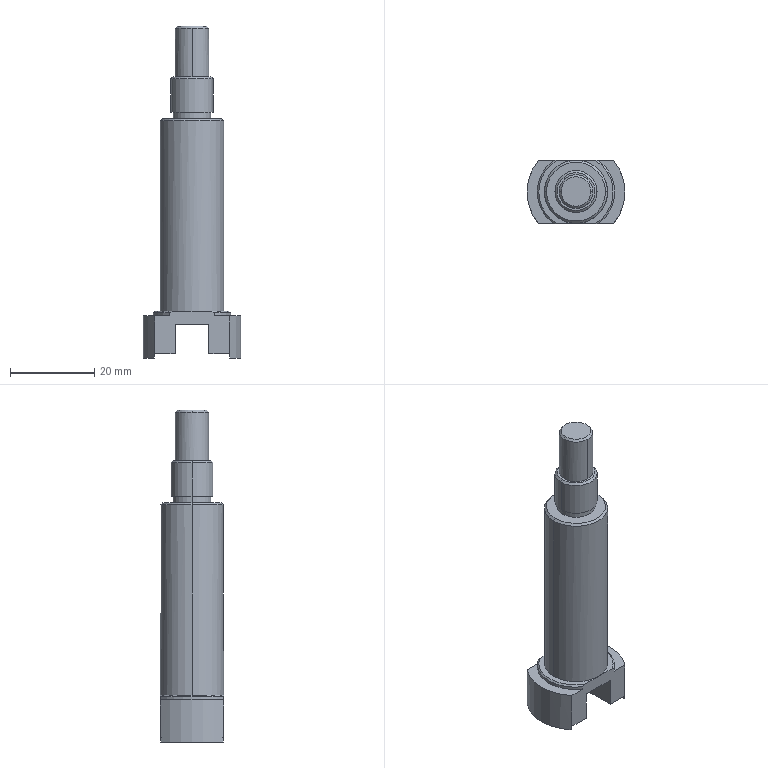Part | NX | 1 solid | 52 faces | box 23.26 x 15 x 78.8 mm | volume 11720 mm3 | plane 19 | cone 17 | cylinder 16 | commonest cylinder face diameters 2.5 x4 8 x2 9 x2 10 x2 15 x2 18.4 x2
STEP:
#1=CARTESIAN_POINT('',(4.5,0.,10.));
#2=VERTEX_POINT('',#1);
#3=CARTESIAN_POINT('',(-4.5,0.,10.));
#4=VERTEX_POINT('',#3);
#5=CARTESIAN_POINT('',(0.,0.,10.));
#6=DIRECTION('',(0.,0.,-1.));
#7=DIRECTION('',(1.,0.,0.));
#8=AXIS2_PLACEMENT_3D('',#5,#6,#7);
#9=CIRCLE('',#8,4.5);
#10=EDGE_CURVE('',#2,#4,#9,.T.);
#11=ORIENTED_EDGE('',*,*,#10,.F.);
#12=CARTESIAN_POINT('',(0.,0.,10.));
#13=DIRECTION('',(0.,0.,-1.));
#14=DIRECTION('',(1.,0.,0.));
#15=AXIS2_PLACEMENT_3D('',#12,#13,#14);
#16=CIRCLE('',#15,4.5);
#17=EDGE_CURVE('',#4,#2,#16,.T.);
#18=ORIENTED_EDGE('',*,*,#17,.F.);
#19=EDGE_LOOP('',(#11,#18));
#20=FACE_BOUND('',#19,.T.);
#21=CARTESIAN_POINT('',(0.,-4.,10.));
#22=VERTEX_POINT('',#21);
#23=CARTESIAN_POINT('',(0.,4.,10.));
#24=VERTEX_POINT('',#23);
#25=CARTESIAN_POINT('',(0.,0.,10.));
#26=DIRECTION('',(0.,0.,1.));
#27=DIRECTION('',(0.,-1.,0.));
#28=AXIS2_PLACEMENT_3D('',#25,#26,#27);
#29=CIRCLE('',#28,4.);
#30=EDGE_CURVE('',#22,#24,#29,.T.);
#31=ORIENTED_EDGE('',*,*,#30,.F.);
#32=CARTESIAN_POINT('',(0.,0.,10.));
#33=DIRECTION('',(0.,0.,1.));
#34=DIRECTION('',(0.,-1.,0.));
#35=AXIS2_PLACEMENT_3D('',#32,#33,#34);
#36=CIRCLE('',#35,4.);
#37=EDGE_CURVE('',#24,#22,#36,.T.);
#38=ORIENTED_EDGE('',*,*,#37,.F.);
#39=EDGE_LOOP('',(#31,#38));
#40=FACE_BOUND('',#39,.T.);
#41=CARTESIAN_POINT('',(0.,0.,10.));
#42=DIRECTION('',(0.,0.,1.));
#43=DIRECTION('',(1.,0.,0.));
#44=AXIS2_PLACEMENT_3D('',#41,#42,#43);
#45=PLANE('',#44);
#46=ADVANCED_FACE('',(#20,#40),#45,.T.);
#47=ORIENTED_EDGE('',*,*,#10,.T.);
#48=CARTESIAN_POINT('',(-5.,0.,9.5));
#49=VERTEX_POINT('',#48);
#50=CARTESIAN_POINT('',(-4.75,0.,9.75));
#51=DIRECTION('',(-0.7071,0.,-0.7071));
#52=VECTOR('',#51,1000.);
#53=LINE('',#50,#52);
#54=EDGE_CURVE('',#49,#4,#53,.F.);
#55=ORIENTED_EDGE('',*,*,#54,.F.);
#56=CARTESIAN_POINT('',(5.,0.,9.5));
#57=VERTEX_POINT('',#56);
#58=CARTESIAN_POINT('',(0.,0.,9.5));
#59=DIRECTION('',(0.,0.,-1.));
#60=DIRECTION('',(1.,0.,0.));
#61=AXIS2_PLACEMENT_3D('',#58,#59,#60);
#62=CIRCLE('',#61,5.);
#63=EDGE_CURVE('',#57,#49,#62,.T.);
#64=ORIENTED_EDGE('',*,*,#63,.F.);
#65=CARTESIAN_POINT('',(4.75,0.,9.75));
#66=DIRECTION('',(0.7071,0.,-0.7071));
#67=VECTOR('',#66,1000.);
#68=LINE('',#65,#67);
#69=EDGE_CURVE('',#57,#2,#68,.F.);
#70=ORIENTED_EDGE('',*,*,#69,.T.);
#71=EDGE_LOOP('',(#47,#55,#64,#70));
#72=FACE_BOUND('',#71,.T.);
#73=CARTESIAN_POINT('',(0.,0.,9.75));
#74=DIRECTION('',(0.,0.,-1.));
#75=DIRECTION('',(-1.,0.,0.));
#76=AXIS2_PLACEMENT_3D('',#73,#74,#75);
#77=CONICAL_SURFACE('',#76,4.75,0.7854);
#78=ADVANCED_FACE('',(#72),#77,.T.);
#79=ORIENTED_EDGE('',*,*,#30,.T.);
#80=CARTESIAN_POINT('',(0.,4.,21.5));
#81=VERTEX_POINT('',#80);
#82=CARTESIAN_POINT('',(0.,4.,10.));
#83=DIRECTION('',(0.,0.,1.));
#84=VECTOR('',#83,1000.);
#85=LINE('',#82,#84);
#86=EDGE_CURVE('',#24,#81,#85,.T.);
#87=ORIENTED_EDGE('',*,*,#86,.T.);
#88=CARTESIAN_POINT('',(4.,0.,21.5));
#89=VERTEX_POINT('',#88);
#90=CARTESIAN_POINT('',(0.,0.,21.5));
#91=DIRECTION('',(0.,0.,-1.));
#92=DIRECTION('',(0.,1.,0.));
#93=AXIS2_PLACEMENT_3D('',#90,#91,#92);
#94=CIRCLE('',#93,4.);
#95=EDGE_CURVE('',#81,#89,#94,.T.);
#96=ORIENTED_EDGE('',*,*,#95,.T.);
#97=CARTESIAN_POINT('',(0.,-4.,21.5));
#98=VERTEX_POINT('',#97);
#99=CARTESIAN_POINT('',(0.,0.,21.5));
#100=DIRECTION('',(0.,0.,-1.));
#101=DIRECTION('',(0.,1.,0.));
#102=AXIS2_PLACEMENT_3D('',#99,#100,#101);
#103=CIRCLE('',#102,4.);
#104=EDGE_CURVE('',#89,#98,#103,.T.);
#105=ORIENTED_EDGE('',*,*,#104,.T.);
#106=CARTESIAN_POINT('',(0.,-4.,10.));
#107=DIRECTION('',(0.,0.,1.));
#108=VECTOR('',#107,1000.);
#109=LINE('',#106,#108);
#110=EDGE_CURVE('',#22,#98,#109,.T.);
#111=ORIENTED_EDGE('',*,*,#110,.F.);
#112=EDGE_LOOP('',(#79,#87,#96,#105,#111));
#113=FACE_BOUND('',#112,.T.);
#114=CARTESIAN_POINT('',(0.,0.,10.));
#115=DIRECTION('',(0.,0.,1.));
#116=DIRECTION('',(0.,1.,0.));
#117=AXIS2_PLACEMENT_3D('',#114,#115,#116);
#118=CYLINDRICAL_SURFACE('',#117,4.);
#119=ADVANCED_FACE('',(#113),#118,.T.);
#120=CARTESIAN_POINT('',(4.8,7.5,-50.8));
#121=VERTEX_POINT('',#120);
#122=CARTESIAN_POINT('',(8.2,7.5,-50.8));
#123=VERTEX_POINT('',#122);
#124=CARTESIAN_POINT('',(6.5,7.5,-50.8));
#125=DIRECTION('',(0.,1.,0.));
#126=DIRECTION('',(1.,0.,0.));
#127=AXIS2_PLACEMENT_3D('',#124,#125,#126);
#128=CIRCLE('',#127,1.7);
#129=EDGE_CURVE('',#121,#123,#128,.T.);
#130=ORIENTED_EDGE('',*,*,#129,.T.);
#131=CARTESIAN_POINT('',(7.75,7.24,-50.8));
#132=VERTEX_POINT('',#131);
#133=CARTESIAN_POINT('',(7.75,7.24,-50.8));
#134=DIRECTION('',(0.866,0.5,0.));
#135=VECTOR('',#134,1000.);
#136=LINE('',#133,#135);
#137=EDGE_CURVE('',#132,#123,#136,.T.);
#138=ORIENTED_EDGE('',*,*,#137,.F.);
#139=CARTESIAN_POINT('',(5.25,7.24,-50.8));
#140=VERTEX_POINT('',#139);
#141=CARTESIAN_POINT('',(6.5,7.24,-50.8));
#142=DIRECTION('',(0.,1.,0.));
#143=DIRECTION('',(1.,0.,0.));
#144=AXIS2_PLACEMENT_3D('',#141,#142,#143);
#145=CIRCLE('',#144,1.25);
#146=EDGE_CURVE('',#140,#132,#145,.T.);
#147=ORIENTED_EDGE('',*,*,#146,.F.);
#148=CARTESIAN_POINT('',(5.25,7.24,-50.8));
#149=DIRECTION('',(-0.866,0.5,0.));
#150=VECTOR('',#149,1000.);
#151=LINE('',#148,#150);
#152=EDGE_CURVE('',#140,#121,#151,.T.);
#153=ORIENTED_EDGE('',*,*,#152,.T.);
#154=EDGE_LOOP('',(#130,#138,#147,#153));
#155=FACE_BOUND('',#154,.T.);
#156=CARTESIAN_POINT('',(6.5,7.24,-50.8));
#157=DIRECTION('',(0.,1.,0.));
#158=DIRECTION('',(1.,0.,0.));
#159=AXIS2_PLACEMENT_3D('',#156,#157,#158);
#160=CONICAL_SURFACE('',#159,1.25,1.047);
#161=ADVANCED_FACE('',(#155),#160,.F.);
#162=ORIENTED_EDGE('',*,*,#63,.T.);
#163=CARTESIAN_POINT('',(-5.,0.,1.5));
#164=VERTEX_POINT('',#163);
#165=CARTESIAN_POINT('',(-5.,0.,0.));
#166=DIRECTION('',(0.,0.,1.));
#167=VECTOR('',#166,1000.);
#168=LINE('',#165,#167);
#169=EDGE_CURVE('',#164,#49,#168,.T.);
#170=ORIENTED_EDGE('',*,*,#169,.F.);
#171=CARTESIAN_POINT('',(5.,0.,1.5));
#172=VERTEX_POINT('',#171);
#173=CARTESIAN_POINT('',(0.,0.,1.5));
#174=DIRECTION('',(0.,0.,1.));
#175=DIRECTION('',(1.,0.,0.));
#176=AXIS2_PLACEMENT_3D('',#173,#174,#175);
#177=CIRCLE('',#176,5.);
#178=EDGE_CURVE('',#164,#172,#177,.T.);
#179=ORIENTED_EDGE('',*,*,#178,.T.);
#180=CARTESIAN_POINT('',(5.,0.,0.));
#181=DIRECTION('',(0.,0.,1.));
#182=VECTOR('',#181,1000.);
#183=LINE('',#180,#182);
#184=EDGE_CURVE('',#172,#57,#183,.T.);
#185=ORIENTED_EDGE('',*,*,#184,.T.);
#186=EDGE_LOOP('',(#162,#170,#179,#185));
#187=FACE_BOUND('',#186,.T.);
#188=CARTESIAN_POINT('',(0.,0.,0.));
#189=DIRECTION('',(0.,0.,1.));
#190=DIRECTION('',(1.,0.,0.));
#191=AXIS2_PLACEMENT_3D('',#188,#189,#190);
#192=CYLINDRICAL_SURFACE('',#191,5.);
#193=ADVANCED_FACE('',(#187),#192,.T.);
#194=CARTESIAN_POINT('',(7.5,0.,-0.5));
#195=VERTEX_POINT('',#194);
#196=CARTESIAN_POINT('',(-7.5,0.,-0.5));
#197=VERTEX_POINT('',#196);
#198=CARTESIAN_POINT('',(0.,0.,-0.5));
#199=DIRECTION('',(0.,0.,-1.));
#200=DIRECTION('',(-1.,0.,0.));
#201=AXIS2_PLACEMENT_3D('',#198,#199,#200);
#202=CIRCLE('',#201,7.5);
#203=EDGE_CURVE('',#195,#197,#202,.T.);
#204=ORIENTED_EDGE('',*,*,#203,.F.);
#205=CARTESIAN_POINT('',(7.,0.,0.));
#206=VERTEX_POINT('',#205);
#207=CARTESIAN_POINT('',(7.25,0.,-0.25));
#208=DIRECTION('',(0.7071,0.,-0.7071));
#209=VECTOR('',#208,1000.);
#210=LINE('',#207,#209);
#211=EDGE_CURVE('',#206,#195,#210,.T.);
#212=ORIENTED_EDGE('',*,*,#211,.F.);
#213=CARTESIAN_POINT('',(-7.,0.,0.));
#214=VERTEX_POINT('',#213);
#215=CARTESIAN_POINT('',(0.,0.,0.));
#216=DIRECTION('',(0.,0.,-1.));
#217=DIRECTION('',(-1.,0.,0.));
#218=AXIS2_PLACEMENT_3D('',#215,#216,#217);
#219=CIRCLE('',#218,7.);
#220=EDGE_CURVE('',#206,#214,#219,.T.);
#221=ORIENTED_EDGE('',*,*,#220,.T.);
#222=CARTESIAN_POINT('',(-7.25,0.,-0.25));
#223=DIRECTION('',(-0.7071,0.,-0.7071));
#224=VECTOR('',#223,1000.);
#225=LINE('',#222,#224);
#226=EDGE_CURVE('',#214,#197,#225,.T.);
#227=ORIENTED_EDGE('',*,*,#226,.T.);
#228=EDGE_LOOP('',(#204,#212,#221,#227));
#229=FACE_BOUND('',#228,.T.);
#230=CARTESIAN_POINT('',(0.,0.,-0.25));
#231=DIRECTION('',(0.,0.,-1.));
#232=DIRECTION('',(-1.,0.,0.));
#233=AXIS2_PLACEMENT_3D('',#230,#231,#232);
#234=CONICAL_SURFACE('',#233,7.25,0.7854);
#235=ADVANCED_FACE('',(#229),#234,.T.);
#236=CARTESIAN_POINT('',(-4.,0.,21.5));
#237=VERTEX_POINT('',#236);
#238=CARTESIAN_POINT('',(0.,0.,21.5));
#239=DIRECTION('',(0.,0.,-1.));
#240=DIRECTION('',(0.,1.,0.));
#241=AXIS2_PLACEMENT_3D('',#238,#239,#240);
#242=CIRCLE('',#241,4.);
#243=EDGE_CURVE('',#237,#81,#242,.T.);
#244=ORIENTED_EDGE('',*,*,#243,.F.);
#245=CARTESIAN_POINT('',(-3.5,0.,22.));
#246=VERTEX_POINT('',#245);
#247=CARTESIAN_POINT('',(-3.75,0.,21.75));
#248=DIRECTION('',(-0.7071,0.,-0.7071));
#249=VECTOR('',#248,1000.);
#250=LINE('',#247,#249);
#251=EDGE_CURVE('',#237,#246,#250,.F.);
#252=ORIENTED_EDGE('',*,*,#251,.T.);
#253=CARTESIAN_POINT('',(3.5,0.,22.));
#254=VERTEX_POINT('',#253);
#255=CARTESIAN_POINT('',(0.,0.,22.));
#256=DIRECTION('',(0.,0.,-1.));
#257=DIRECTION('',(0.,-1.,0.));
#258=AXIS2_PLACEMENT_3D('',#255,#256,#257);
#259=CIRCLE('',#258,3.5);
#260=EDGE_CURVE('',#246,#254,#259,.T.);
#261=ORIENTED_EDGE('',*,*,#260,.T.);
#262=CARTESIAN_POINT('',(3.75,0.,21.75));
#263=DIRECTION('',(0.7071,0.,-0.7071));
#264=VECTOR('',#263,1000.);
#265=LINE('',#262,#264);
#266=EDGE_CURVE('',#89,#254,#265,.F.);
#267=ORIENTED_EDGE('',*,*,#266,.F.);
#268=ORIENTED_EDGE('',*,*,#95,.F.);
#269=EDGE_LOOP('',(#244,#252,#261,#267,#268));
#270=FACE_BOUND('',#269,.T.);
#271=CARTESIAN_POINT('',(0.,0.,21.75));
#272=DIRECTION('',(0.,0.,-1.));
#273=DIRECTION('',(-1.,0.,0.));
#274=AXIS2_PLACEMENT_3D('',#271,#272,#273);
#275=CONICAL_SURFACE('',#274,3.75,0.7854);
#276=ADVANCED_FACE('',(#270),#275,.T.);
#277=ORIENTED_EDGE('',*,*,#203,.T.);
#278=CARTESIAN_POINT('',(-7.5,0.,-45.7));
#279=VERTEX_POINT('',#278);
#280=CARTESIAN_POINT('',(-7.5,0.,2.34));
#281=DIRECTION('',(0.,0.,-1.));
#282=VECTOR('',#281,1000.);
#283=LINE('',#280,#282);
#284=EDGE_CURVE('',#279,#197,#283,.F.);
#285=ORIENTED_EDGE('',*,*,#284,.F.);
#286=CARTESIAN_POINT('',(0.,-7.5,-45.7));
#287=VERTEX_POINT('',#286);
#288=CARTESIAN_POINT('',(0.,0.,-45.7));
#289=DIRECTION('',(0.,0.,1.));
#290=DIRECTION('',(-1.,0.,0.));
#291=AXIS2_PLACEMENT_3D('',#288,#289,#290);
#292=CIRCLE('',#291,7.5);
#293=EDGE_CURVE('',#279,#287,#292,.T.);
#294=ORIENTED_EDGE('',*,*,#293,.T.);
#295=CARTESIAN_POINT('',(7.5,0.,-45.7));
#296=VERTEX_POINT('',#295);
#297=CARTESIAN_POINT('',(0.,0.,-45.7));
#298=DIRECTION('',(0.,0.,1.));
#299=DIRECTION('',(0.,-1.,0.));
#300=AXIS2_PLACEMENT_3D('',#297,#298,#299);
#301=CIRCLE('',#300,7.5);
#302=EDGE_CURVE('',#287,#296,#301,.T.);
#303=ORIENTED_EDGE('',*,*,#302,.T.);
#304=CARTESIAN_POINT('',(7.5,0.,2.34));
#305=DIRECTION('',(0.,0.,-1.));
#306=VECTOR('',#305,1000.);
#307=LINE('',#304,#306);
#308=EDGE_CURVE('',#296,#195,#307,.F.);
#309=ORIENTED_EDGE('',*,*,#308,.T.);
#310=EDGE_LOOP('',(#277,#285,#294,#303,#309));
#311=FACE_BOUND('',#310,.T.);
#312=CARTESIAN_POINT('',(0.,0.,2.34));
#313=DIRECTION('',(0.,0.,-1.));
#314=DIRECTION('',(1.,0.,0.));
#315=AXIS2_PLACEMENT_3D('',#312,#313,#314);
#316=CYLINDRICAL_SURFACE('',#315,7.5);
#317=ADVANCED_FACE('',(#311),#316,.T.);
#318=CARTESIAN_POINT('',(-4.651,7.5,-45.7));
#319=VERTEX_POINT('',#318);
#320=CARTESIAN_POINT('',(0.,7.5,-45.7));
#321=VERTEX_POINT('',#320);
#322=CARTESIAN_POINT('',(0.,7.5,-45.7));
#323=DIRECTION('',(1.,0.,0.));
#324=VECTOR('',#323,1000.);
#325=LINE('',#322,#324);
#326=EDGE_CURVE('',#319,#321,#325,.T.);
#327=ORIENTED_EDGE('',*,*,#326,.F.);
#328=CARTESIAN_POINT('',(-8.825,0.,-45.7));
#329=VERTEX_POINT('',#328);
#330=CARTESIAN_POINT('',(0.,0.,-45.7));
#331=DIRECTION('',(0.,0.,-1.));
#332=DIRECTION('',(-1.,0.,0.));
#333=AXIS2_PLACEMENT_3D('',#330,#331,#332);
#334=CIRCLE('',#333,8.825);
#335=EDGE_CURVE('',#329,#319,#334,.T.);
#336=ORIENTED_EDGE('',*,*,#335,.F.);
#337=CARTESIAN_POINT('',(-4.651,-7.5,-45.7));
#338=VERTEX_POINT('',#337);
#339=CARTESIAN_POINT('',(0.,0.,-45.7));
#340=DIRECTION('',(0.,0.,-1.));
#341=DIRECTION('',(-1.,0.,0.));
#342=AXIS2_PLACEMENT_3D('',#339,#340,#341);
#343=CIRCLE('',#342,8.825);
#344=EDGE_CURVE('',#338,#329,#343,.T.);
#345=ORIENTED_EDGE('',*,*,#344,.F.);
#346=CARTESIAN_POINT('',(0.,-7.5,-45.7));
#347=DIRECTION('',(-1.,0.,0.));
#348=VECTOR('',#347,1000.);
#349=LINE('',#346,#348);
#350=EDGE_CURVE('',#287,#338,#349,.T.);
#351=ORIENTED_EDGE('',*,*,#350,.F.);
#352=ORIENTED_EDGE('',*,*,#293,.F.);
#353=CARTESIAN_POINT('',(0.,0.,-45.7));
#354=DIRECTION('',(0.,0.,1.));
#355=DIRECTION('',(-1.,0.,0.));
#356=AXIS2_PLACEMENT_3D('',#353,#354,#355);
#357=CIRCLE('',#356,7.5);
#358=EDGE_CURVE('',#321,#279,#357,.T.);
#359=ORIENTED_EDGE('',*,*,#358,.F.);
#360=EDGE_LOOP('',(#327,#336,#345,#351,#352,#359));
#361=FACE_BOUND('',#360,.T.);
#362=CARTESIAN_POINT('',(0.,0.,-45.7));
#363=DIRECTION('',(0.,0.,1.));
#364=DIRECTION('',(1.,0.,0.));
#365=AXIS2_PLACEMENT_3D('',#362,#363,#364);
#366=PLANE('',#365);
#367=ADVANCED_FACE('',(#361),#366,.T.);
#368=CARTESIAN_POINT('',(4.,7.5,-55.8));
#369=VERTEX_POINT('',#368);
#370=CARTESIAN_POINT('',(8.889,7.5,-55.8));
#371=VERTEX_POINT('',#370);
#372=CARTESIAN_POINT('',(0.,7.5,-55.8));
#373=DIRECTION('',(1.,0.,0.));
#374=VECTOR('',#373,1000.);
#375=LINE('',#372,#374);
#376=EDGE_CURVE('',#369,#371,#375,.T.);
#377=ORIENTED_EDGE('',*,*,#376,.F.);
#378=CARTESIAN_POINT('',(4.,7.5,-48.8));
#379=VERTEX_POINT('',#378);
#380=CARTESIAN_POINT('',(4.,7.5,0.));
#381=DIRECTION('',(0.,0.,-1.));
#382=VECTOR('',#381,1000.);
#383=LINE('',#380,#382);
#384=EDGE_CURVE('',#379,#369,#383,.T.);
#385=ORIENTED_EDGE('',*,*,#384,.F.);
#386=CARTESIAN_POINT('',(-4.,7.5,-48.8));
#387=VERTEX_POINT('',#386);
#388=CARTESIAN_POINT('',(0.,7.5,-48.8));
#389=DIRECTION('',(1.,0.,0.));
#390=VECTOR('',#389,1000.);
#391=LINE('',#388,#390);
#392=EDGE_CURVE('',#387,#379,#391,.T.);
#393=ORIENTED_EDGE('',*,*,#392,.F.);
#394=CARTESIAN_POINT('',(-4.,7.5,-55.8));
#395=VERTEX_POINT('',#394);
#396=CARTESIAN_POINT('',(-4.,7.5,0.));
#397=DIRECTION('',(0.,0.,1.));
#398=VECTOR('',#397,1000.);
#399=LINE('',#396,#398);
#400=EDGE_CURVE('',#395,#387,#399,.T.);
#401=ORIENTED_EDGE('',*,*,#400,.F.);
#402=CARTESIAN_POINT('',(-8.889,7.5,-55.8));
#403=VERTEX_POINT('',#402);
#404=CARTESIAN_POINT('',(0.,7.5,-55.8));
#405=DIRECTION('',(1.,0.,0.));
#406=VECTOR('',#405,1000.);
#407=LINE('',#404,#406);
#408=EDGE_CURVE('',#403,#395,#407,.T.);
#409=ORIENTED_EDGE('',*,*,#408,.F.);
#410=CARTESIAN_POINT('',(-8.889,7.5,-46.8));
#411=VERTEX_POINT('',#410);
#412=CARTESIAN_POINT('',(-8.889,7.5,0.));
#413=DIRECTION('',(0.,0.,-1.));
#414=VECTOR('',#413,1000.);
#415=LINE('',#412,#414);
#416=EDGE_CURVE('',#411,#403,#415,.T.);
#417=ORIENTED_EDGE('',*,*,#416,.F.);
#418=CARTESIAN_POINT('',(-5.328,7.5,-46.8));
#419=VERTEX_POINT('',#418);
#420=CARTESIAN_POINT('',(0.,7.5,-46.8));
#421=DIRECTION('',(-1.,0.,0.));
#422=VECTOR('',#421,1000.);
#423=LINE('',#420,#422);
#424=EDGE_CURVE('',#419,#411,#423,.T.);
#425=ORIENTED_EDGE('',*,*,#424,.F.);
#426=CARTESIAN_POINT('',(-5.328,7.5,-46.075));
#427=VERTEX_POINT('',#426);
#428=CARTESIAN_POINT('',(-5.328,7.5,-46.8));
#429=DIRECTION('',(0.,0.,1.));
#430=VECTOR('',#429,1000.);
#431=LINE('',#428,#430);
#432=EDGE_CURVE('',#419,#427,#431,.T.);
#433=ORIENTED_EDGE('',*,*,#432,.T.);
#434=CARTESIAN_POINT('',(-5.328,7.5,-46.075));
#435=CARTESIAN_POINT('',(-5.273,7.5,-46.043));
#436=CARTESIAN_POINT('',(-5.217,7.5,-46.011));
#437=CARTESIAN_POINT('',(-5.161,7.5,-45.979));
#438=CARTESIAN_POINT('',(-5.104,7.5,-45.947));
#439=CARTESIAN_POINT('',(-5.048,7.5,-45.916));
#440=CARTESIAN_POINT('',(-4.992,7.5,-45.884));
#441=CARTESIAN_POINT('',(-4.935,7.5,-45.853));
#442=CARTESIAN_POINT('',(-4.879,7.5,-45.822));
#443=CARTESIAN_POINT('',(-4.822,7.5,-45.791));
#444=CARTESIAN_POINT('',(-4.765,7.5,-45.761));
#445=CARTESIAN_POINT('',(-4.708,7.5,-45.73));
#446=CARTESIAN_POINT('',(-4.651,7.5,-45.7));
#447=B_SPLINE_CURVE_WITH_KNOTS('',3,(#434,#435,#436,#437,#438,#439,#440,#441,#442,#443,#444,#445,#446),.UNSPECIFIED.,.F.,.F.,(4,3,3,3,4),(0.,0.1932,0.3867,0.5804,0.7743),.UNSPECIFIED.);
#448=EDGE_CURVE('',#427,#319,#447,.T.);
#449=ORIENTED_EDGE('',*,*,#448,.T.);
#450=ORIENTED_EDGE('',*,*,#326,.T.);
#451=CARTESIAN_POINT('',(4.651,7.5,-45.7));
#452=VERTEX_POINT('',#451);
#453=CARTESIAN_POINT('',(0.,7.5,-45.7));
#454=DIRECTION('',(1.,0.,0.));
#455=VECTOR('',#454,1000.);
#456=LINE('',#453,#455);
#457=EDGE_CURVE('',#321,#452,#456,.T.);
#458=ORIENTED_EDGE('',*,*,#457,.T.);
#459=CARTESIAN_POINT('',(5.328,7.5,-46.075));
#460=VERTEX_POINT('',#459);
#461=CARTESIAN_POINT('',(4.651,7.5,-45.7));
#462=CARTESIAN_POINT('',(4.708,7.5,-45.73));
#463=CARTESIAN_POINT('',(4.765,7.5,-45.761));
#464=CARTESIAN_POINT('',(4.822,7.5,-45.791));
#465=CARTESIAN_POINT('',(4.879,7.5,-45.822));
#466=CARTESIAN_POINT('',(4.935,7.5,-45.853));
#467=CARTESIAN_POINT('',(4.992,7.5,-45.884));
#468=CARTESIAN_POINT('',(5.048,7.5,-45.916));
#469=CARTESIAN_POINT('',(5.104,7.5,-45.947));
#470=CARTESIAN_POINT('',(5.161,7.5,-45.979));
#471=CARTESIAN_POINT('',(5.217,7.5,-46.011));
#472=CARTESIAN_POINT('',(5.273,7.5,-46.043));
#473=CARTESIAN_POINT('',(5.328,7.5,-46.075));
#474=B_SPLINE_CURVE_WITH_KNOTS('',3,(#461,#462,#463,#464,#465,#466,#467,#468,#469,#470,#471,#472,#473),.UNSPECIFIED.,.F.,.F.,(4,3,3,3,4),(0.,0.1939,0.3875,0.581,0.7743),.UNSPECIFIED.);
#475=EDGE_CURVE('',#452,#460,#474,.T.);
#476=ORIENTED_EDGE('',*,*,#475,.T.);
#477=CARTESIAN_POINT('',(5.328,7.5,-46.8));
#478=VERTEX_POINT('',#477);
#479=CARTESIAN_POINT('',(5.328,7.5,-46.8));
#480=DIRECTION('',(0.,0.,1.));
#481=VECTOR('',#480,1000.);
#482=LINE('',#479,#481);
#483=EDGE_CURVE('',#478,#460,#482,.T.);
#484=ORIENTED_EDGE('',*,*,#483,.F.);
#485=CARTESIAN_POINT('',(8.889,7.5,-46.8));
#486=VERTEX_POINT('',#485);
#487=CARTESIAN_POINT('',(0.,7.5,-46.8));
#488=DIRECTION('',(1.,0.,0.));
#489=VECTOR('',#488,1000.);
#490=LINE('',#487,#489);
#491=EDGE_CURVE('',#478,#486,#490,.T.);
#492=ORIENTED_EDGE('',*,*,#491,.T.);
#493=CARTESIAN_POINT('',(8.889,7.5,0.));
#494=DIRECTION('',(0.,0.,-1.));
#495=VECTOR('',#494,1000.);
#496=LINE('',#493,#495);
#497=EDGE_CURVE('',#486,#371,#496,.T.);
#498=ORIENTED_EDGE('',*,*,#497,.T.);
#499=EDGE_LOOP('',(#377,#385,#393,#401,#409,#417,#425,#433,#449,#450,#458,#476,#484,#492,#498));
#500=FACE_BOUND('',#499,.T.);
#501=CARTESIAN_POINT('',(-8.2,7.5,-50.8));
#502=VERTEX_POINT('',#501);
#503=CARTESIAN_POINT('',(-4.8,7.5,-50.8));
#504=VERTEX_POINT('',#503);
#505=CARTESIAN_POINT('',(-6.5,7.5,-50.8));
#506=DIRECTION('',(0.,1.,0.));
#507=DIRECTION('',(1.,0.,0.));
#508=AXIS2_PLACEMENT_3D('',#505,#506,#507);
#509=CIRCLE('',#508,1.7);
#510=EDGE_CURVE('',#502,#504,#509,.T.);
#511=ORIENTED_EDGE('',*,*,#510,.F.);
#512=CARTESIAN_POINT('',(-6.5,7.5,-50.8));
#513=DIRECTION('',(0.,1.,0.));
#514=DIRECTION('',(1.,0.,0.));
#515=AXIS2_PLACEMENT_3D('',#512,#513,#514);
#516=CIRCLE('',#515,1.7);
#517=EDGE_CURVE('',#504,#502,#516,.T.);
#518=ORIENTED_EDGE('',*,*,#517,.F.);
#519=EDGE_LOOP('',(#511,#518));
#520=FACE_BOUND('',#519,.T.);
#521=ORIENTED_EDGE('',*,*,#129,.F.);
#522=CARTESIAN_POINT('',(6.5,7.5,-50.8));
#523=DIRECTION('',(0.,1.,0.));
#524=DIRECTION('',(1.,0.,0.));
#525=AXIS2_PLACEMENT_3D('',#522,#523,#524);
#526=CIRCLE('',#525,1.7);
#527=EDGE_CURVE('',#123,#121,#526,.T.);
#528=ORIENTED_EDGE('',*,*,#527,.F.);
#529=EDGE_LOOP('',(#521,#528));
#530=FACE_BOUND('',#529,.T.);
#531=CARTESIAN_POINT('',(10.579,7.5,-56.8));
#532=DIRECTION('',(0.,-1.,0.));
#533=DIRECTION('',(0.,0.,-1.));
#534=AXIS2_PLACEMENT_3D('',#531,#532,#533);
#535=PLANE('',#534);
#536=ADVANCED_FACE('',(#500,#520,#530),#535,.F.);
#537=ORIENTED_EDGE('',*,*,#376,.T.);
#538=CARTESIAN_POINT('',(9.,7.366,-55.8));
#539=VERTEX_POINT('',#538);
#540=CARTESIAN_POINT('',(0.,0.,-55.8));
#541=DIRECTION('',(0.,0.,-1.));
#542=DIRECTION('',(0.,-1.,0.));
#543=AXIS2_PLACEMENT_3D('',#540,#541,#542);
#544=CIRCLE('',#543,11.63);
#545=EDGE_CURVE('',#371,#539,#544,.T.);
#546=ORIENTED_EDGE('',*,*,#545,.T.);
#547=CARTESIAN_POINT('',(9.,-7.366,-55.8));
#548=VERTEX_POINT('',#547);
#549=CARTESIAN_POINT('',(9.,0.,-55.8));
#550=DIRECTION('',(0.,1.,0.));
#551=VECTOR('',#550,1000.);
#552=LINE('',#549,#551);
#553=EDGE_CURVE('',#548,#539,#552,.T.);
#554=ORIENTED_EDGE('',*,*,#553,.F.);
#555=CARTESIAN_POINT('',(8.889,-7.5,-55.8));
#556=VERTEX_POINT('',#555);
#557=CARTESIAN_POINT('',(0.,0.,-55.8));
#558=DIRECTION('',(0.,0.,-1.));
#559=DIRECTION('',(0.,-1.,0.));
#560=AXIS2_PLACEMENT_3D('',#557,#558,#559);
#561=CIRCLE('',#560,11.63);
#562=EDGE_CURVE('',#548,#556,#561,.T.);
#563=ORIENTED_EDGE('',*,*,#562,.T.);
#564=CARTESIAN_POINT('',(4.,-7.5,-55.8));
#565=VERTEX_POINT('',#564);
#566=CARTESIAN_POINT('',(0.,-7.5,-55.8));
#567=DIRECTION('',(-1.,0.,0.));
#568=VECTOR('',#567,1000.);
#569=LINE('',#566,#568);
#570=EDGE_CURVE('',#556,#565,#569,.T.);
#571=ORIENTED_EDGE('',*,*,#570,.T.);
#572=CARTESIAN_POINT('',(4.,0.,-55.8));
#573=DIRECTION('',(0.,-1.,0.));
#574=VECTOR('',#573,1000.);
#575=LINE('',#572,#574);
#576=EDGE_CURVE('',#369,#565,#575,.T.);
#577=ORIENTED_EDGE('',*,*,#576,.F.);
#578=EDGE_LOOP('',(#537,#546,#554,#563,#571,#577));
#579=FACE_BOUND('',#578,.T.);
#580=CARTESIAN_POINT('',(-9.,7.5,-55.8));
#581=DIRECTION('',(0.,0.,1.));
#582=DIRECTION('',(1.,0.,0.));
#583=AXIS2_PLACEMENT_3D('',#580,#581,#582);
#584=PLANE('',#583);
#585=ADVANCED_FACE('',(#579),#584,.F.);
#586=ORIENTED_EDGE('',*,*,#576,.T.);
#587=CARTESIAN_POINT('',(4.,-7.5,-48.8));
#588=VERTEX_POINT('',#587);
#589=CARTESIAN_POINT('',(4.,-7.5,0.));
#590=DIRECTION('',(0.,0.,1.));
#591=VECTOR('',#590,1000.);
#592=LINE('',#589,#591);
#593=EDGE_CURVE('',#565,#588,#592,.T.);
#594=ORIENTED_EDGE('',*,*,#593,.T.);
#595=CARTESIAN_POINT('',(4.,-7.5,-48.8));
#596=DIRECTION('',(0.,1.,0.));
#597=VECTOR('',#596,1000.);
#598=LINE('',#595,#597);
#599=EDGE_CURVE('',#588,#379,#598,.T.);
#600=ORIENTED_EDGE('',*,*,#599,.T.);
#601=ORIENTED_EDGE('',*,*,#384,.T.);
#602=EDGE_LOOP('',(#586,#594,#600,#601));
#603=FACE_BOUND('',#602,.T.);
#604=CARTESIAN_POINT('',(4.,7.5,-48.8));
#605=DIRECTION('',(1.,0.,0.));
#606=DIRECTION('',(0.,1.,0.));
#607=AXIS2_PLACEMENT_3D('',#604,#605,#606);
#608=PLANE('',#607);
#609=ADVANCED_FACE('',(#603),#608,.F.);
#610=CARTESIAN_POINT('',(-4.,-7.5,-48.8));
#611=VERTEX_POINT('',#610);
#612=CARTESIAN_POINT('',(-4.,-7.5,-48.8));
#613=DIRECTION('',(0.,1.,0.));
#614=VECTOR('',#613,1000.);
#615=LINE('',#612,#614);
#616=EDGE_CURVE('',#611,#387,#615,.T.);
#617=ORIENTED_EDGE('',*,*,#616,.T.);
#618=ORIENTED_EDGE('',*,*,#392,.T.);
#619=ORIENTED_EDGE('',*,*,#599,.F.);
#620=CARTESIAN_POINT('',(0.,-7.5,-48.8));
#621=DIRECTION('',(-1.,0.,0.));
#622=VECTOR('',#621,1000.);
#623=LINE('',#620,#622);
#624=EDGE_CURVE('',#588,#611,#623,.T.);
#625=ORIENTED_EDGE('',*,*,#624,.T.);
#626=EDGE_LOOP('',(#617,#618,#619,#625));
#627=FACE_BOUND('',#626,.T.);
#628=CARTESIAN_POINT('',(-4.,7.5,-48.8));
#629=DIRECTION('',(0.,0.,1.));
#630=DIRECTION('',(1.,0.,0.));
#631=AXIS2_PLACEMENT_3D('',#628,#629,#630);
#632=PLANE('',#631);
#633=ADVANCED_FACE('',(#627),#632,.F.);
#634=CARTESIAN_POINT('',(-4.,-7.5,-55.8));
#635=VERTEX_POINT('',#634);
#636=CARTESIAN_POINT('',(-4.,0.,-55.8));
#637=DIRECTION('',(0.,1.,0.));
#638=VECTOR('',#637,1000.);
#639=LINE('',#636,#638);
#640=EDGE_CURVE('',#635,#395,#639,.T.);
#641=ORIENTED_EDGE('',*,*,#640,.T.);
#642=ORIENTED_EDGE('',*,*,#400,.T.);
#643=ORIENTED_EDGE('',*,*,#616,.F.);
#644=CARTESIAN_POINT('',(-4.,-7.5,0.));
#645=DIRECTION('',(0.,0.,-1.));
#646=VECTOR('',#645,1000.);
#647=LINE('',#644,#646);
#648=EDGE_CURVE('',#611,#635,#647,.T.);
#649=ORIENTED_EDGE('',*,*,#648,.T.);
#650=EDGE_LOOP('',(#641,#642,#643,#649));
#651=FACE_BOUND('',#650,.T.);
#652=CARTESIAN_POINT('',(-4.,7.5,-56.8));
#653=DIRECTION('',(-1.,0.,0.));
#654=DIRECTION('',(0.,0.,1.));
#655=AXIS2_PLACEMENT_3D('',#652,#653,#654);
#656=PLANE('',#655);
#657=ADVANCED_FACE('',(#651),#656,.F.);
#658=ORIENTED_EDGE('',*,*,#408,.T.);
#659=ORIENTED_EDGE('',*,*,#640,.F.);
#660=CARTESIAN_POINT('',(-8.889,-7.5,-55.8));
#661=VERTEX_POINT('',#660);
#662=CARTESIAN_POINT('',(0.,-7.5,-55.8));
#663=DIRECTION('',(-1.,0.,0.));
#664=VECTOR('',#663,1000.);
#665=LINE('',#662,#664);
#666=EDGE_CURVE('',#635,#661,#665,.T.);
#667=ORIENTED_EDGE('',*,*,#666,.T.);
#668=CARTESIAN_POINT('',(-9.,-7.366,-55.8));
#669=VERTEX_POINT('',#668);
#670=CARTESIAN_POINT('',(0.,0.,-55.8));
#671=DIRECTION('',(0.,0.,-1.));
#672=DIRECTION('',(0.,-1.,0.));
#673=AXIS2_PLACEMENT_3D('',#670,#671,#672);
#674=CIRCLE('',#673,11.63);
#675=EDGE_CURVE('',#661,#669,#674,.T.);
#676=ORIENTED_EDGE('',*,*,#675,.T.);
#677=CARTESIAN_POINT('',(-9.,7.366,-55.8));
#678=VERTEX_POINT('',#677);
#679=CARTESIAN_POINT('',(-9.,0.,-55.8));
#680=DIRECTION('',(0.,1.,0.));
#681=VECTOR('',#680,1000.);
#682=LINE('',#679,#681);
#683=EDGE_CURVE('',#669,#678,#682,.T.);
#684=ORIENTED_EDGE('',*,*,#683,.T.);
#685=CARTESIAN_POINT('',(0.,0.,-55.8));
#686=DIRECTION('',(0.,0.,-1.));
#687=DIRECTION('',(0.,-1.,0.));
#688=AXIS2_PLACEMENT_3D('',#685,#686,#687);
#689=CIRCLE('',#688,11.63);
#690=EDGE_CURVE('',#678,#403,#689,.T.);
#691=ORIENTED_EDGE('',*,*,#690,.T.);
#692=EDGE_LOOP('',(#658,#659,#667,#676,#684,#691));
#693=FACE_BOUND('',#692,.T.);
#694=CARTESIAN_POINT('',(-9.,7.5,-55.8));
#695=DIRECTION('',(0.,0.,1.));
#696=DIRECTION('',(1.,0.,0.));
#697=AXIS2_PLACEMENT_3D('',#694,#695,#696);
#698=PLANE('',#697);
#699=ADVANCED_FACE('',(#693),#698,.F.);
#700=CARTESIAN_POINT('',(-9.,-7.366,-56.8));
#701=VERTEX_POINT('',#700);
#702=CARTESIAN_POINT('',(-9.,-7.366,0.));
#703=DIRECTION('',(0.,0.,-1.));
#704=VECTOR('',#703,1000.);
#705=LINE('',#702,#704);
#706=EDGE_CURVE('',#669,#701,#705,.T.);
#707=ORIENTED_EDGE('',*,*,#706,.F.);
#708=ORIENTED_EDGE('',*,*,#675,.F.);
#709=CARTESIAN_POINT('',(-8.889,-7.5,-46.8));
#710=VERTEX_POINT('',#709);
#711=CARTESIAN_POINT('',(-8.889,-7.5,0.));
#712=DIRECTION('',(0.,0.,-1.));
#713=VECTOR('',#712,1000.);
#714=LINE('',#711,#713);
#715=EDGE_CURVE('',#710,#661,#714,.T.);
#716=ORIENTED_EDGE('',*,*,#715,.F.);
#717=CARTESIAN_POINT('',(0.,0.,-46.8));
#718=DIRECTION('',(0.,0.,-1.));
#719=DIRECTION('',(0.,-1.,0.));
#720=AXIS2_PLACEMENT_3D('',#717,#718,#719);
#721=CIRCLE('',#720,11.63);
#722=EDGE_CURVE('',#710,#411,#721,.T.);
#723=ORIENTED_EDGE('',*,*,#722,.T.);
#724=ORIENTED_EDGE('',*,*,#416,.T.);
#725=ORIENTED_EDGE('',*,*,#690,.F.);
#726=CARTESIAN_POINT('',(-9.,7.366,-56.8));
#727=VERTEX_POINT('',#726);
#728=CARTESIAN_POINT('',(-9.,7.366,0.));
#729=DIRECTION('',(0.,0.,-1.));
#730=VECTOR('',#729,1000.);
#731=LINE('',#728,#730);
#732=EDGE_CURVE('',#678,#727,#731,.T.);
#733=ORIENTED_EDGE('',*,*,#732,.T.);
#734=CARTESIAN_POINT('',(0.,0.,-56.8));
#735=DIRECTION('',(0.,0.,-1.));
#736=DIRECTION('',(0.,-1.,0.));
#737=AXIS2_PLACEMENT_3D('',#734,#735,#736);
#738=CIRCLE('',#737,11.63);
#739=EDGE_CURVE('',#701,#727,#738,.T.);
#740=ORIENTED_EDGE('',*,*,#739,.F.);
#741=EDGE_LOOP('',(#707,#708,#716,#723,#724,#725,#733,#740));
#742=FACE_BOUND('',#741,.T.);
#743=CARTESIAN_POINT('',(0.,0.,0.));
#744=DIRECTION('',(0.,0.,-1.));
#745=DIRECTION('',(0.,-1.,0.));
#746=AXIS2_PLACEMENT_3D('',#743,#744,#745);
#747=CYLINDRICAL_SURFACE('',#746,11.63);
#748=ADVANCED_FACE('',(#742),#747,.T.);
#749=CARTESIAN_POINT('',(-9.,0.,-56.8));
#750=DIRECTION('',(0.,-1.,0.));
#751=VECTOR('',#750,1000.);
#752=LINE('',#749,#751);
#753=EDGE_CURVE('',#727,#701,#752,.T.);
#754=ORIENTED_EDGE('',*,*,#753,.F.);
#755=ORIENTED_EDGE('',*,*,#732,.F.);
#756=ORIENTED_EDGE('',*,*,#683,.F.);
#757=ORIENTED_EDGE('',*,*,#706,.T.);
#758=EDGE_LOOP('',(#754,#755,#756,#757));
#759=FACE_BOUND('',#758,.T.);
#760=CARTESIAN_POINT('',(-9.,7.5,-56.8));
#761=DIRECTION('',(-1.,0.,0.));
#762=DIRECTION('',(0.,0.,1.));
#763=AXIS2_PLACEMENT_3D('',#760,#761,#762);
#764=PLANE('',#763);
#765=ADVANCED_FACE('',(#759),#764,.F.);
#766=ORIENTED_EDGE('',*,*,#753,.T.);
#767=ORIENTED_EDGE('',*,*,#739,.T.);
#768=EDGE_LOOP('',(#766,#767));
#769=FACE_BOUND('',#768,.T.);
#770=CARTESIAN_POINT('',(-7.5,7.,-56.8));
#771=DIRECTION('',(0.,0.,1.));
#772=DIRECTION('',(1.,0.,0.));
#773=AXIS2_PLACEMENT_3D('',#770,#771,#772);
#774=PLANE('',#773);
#775=ADVANCED_FACE('',(#769),#774,.F.);
#776=ORIENTED_EDGE('',*,*,#424,.T.);
#777=ORIENTED_EDGE('',*,*,#722,.F.);
#778=CARTESIAN_POINT('',(-5.328,-7.5,-46.8));
#779=VERTEX_POINT('',#778);
#780=CARTESIAN_POINT('',(0.,-7.5,-46.8));
#781=DIRECTION('',(1.,0.,0.));
#782=VECTOR('',#781,1000.);
#783=LINE('',#780,#782);
#784=EDGE_CURVE('',#710,#779,#783,.T.);
#785=ORIENTED_EDGE('',*,*,#784,.T.);
#786=CARTESIAN_POINT('',(0.,0.,-46.8));
#787=DIRECTION('',(0.,0.,1.));
#788=DIRECTION('',(0.,-1.,0.));
#789=AXIS2_PLACEMENT_3D('',#786,#787,#788);
#790=CIRCLE('',#789,9.2);
#791=EDGE_CURVE('',#419,#779,#790,.T.);
#792=ORIENTED_EDGE('',*,*,#791,.F.);
#793=EDGE_LOOP('',(#776,#777,#785,#792));
#794=FACE_BOUND('',#793,.T.);
#795=CARTESIAN_POINT('',(0.,0.,-46.8));
#796=DIRECTION('',(0.,0.,-1.));
#797=DIRECTION('',(0.,-1.,0.));
#798=AXIS2_PLACEMENT_3D('',#795,#796,#797);
#799=PLANE('',#798);
#800=ADVANCED_FACE('',(#794),#799,.F.);
#801=ORIENTED_EDGE('',*,*,#432,.F.);
#802=ORIENTED_EDGE('',*,*,#791,.T.);
#803=CARTESIAN_POINT('',(-5.328,-7.5,-46.075));
#804=VERTEX_POINT('',#803);
#805=CARTESIAN_POINT('',(-5.328,-7.5,-46.8));
#806=DIRECTION('',(0.,0.,1.));
#807=VECTOR('',#806,1000.);
#808=LINE('',#805,#807);
#809=EDGE_CURVE('',#779,#804,#808,.T.);
#810=ORIENTED_EDGE('',*,*,#809,.T.);
#811=CARTESIAN_POINT('',(-9.2,0.,-46.075));
#812=VERTEX_POINT('',#811);
#813=CARTESIAN_POINT('',(0.,0.,-46.075));
#814=DIRECTION('',(0.,0.,-1.));
#815=DIRECTION('',(-1.,0.,0.));
#816=AXIS2_PLACEMENT_3D('',#813,#814,#815);
#817=CIRCLE('',#816,9.2);
#818=EDGE_CURVE('',#804,#812,#817,.T.);
#819=ORIENTED_EDGE('',*,*,#818,.T.);
#820=CARTESIAN_POINT('',(0.,0.,-46.075));
#821=DIRECTION('',(0.,0.,-1.));
#822=DIRECTION('',(-1.,0.,0.));
#823=AXIS2_PLACEMENT_3D('',#820,#821,#822);
#824=CIRCLE('',#823,9.2);
#825=EDGE_CURVE('',#812,#427,#824,.T.);
#826=ORIENTED_EDGE('',*,*,#825,.T.);
#827=EDGE_LOOP('',(#801,#802,#810,#819,#826));
#828=FACE_BOUND('',#827,.T.);
#829=CARTESIAN_POINT('',(0.,0.,-46.8));
#830=DIRECTION('',(0.,0.,1.));
#831=DIRECTION('',(0.,-1.,0.));
#832=AXIS2_PLACEMENT_3D('',#829,#830,#831);
#833=CYLINDRICAL_SURFACE('',#832,9.2);
#834=ADVANCED_FACE('',(#828),#833,.T.);
#835=CARTESIAN_POINT('',(-8.975,0.,-45.85));
#836=DIRECTION('',(-0.7071,0.,-0.7071));
#837=VECTOR('',#836,1000.);
#838=LINE('',#835,#837);
#839=EDGE_CURVE('',#329,#812,#838,.T.);
#840=ORIENTED_EDGE('',*,*,#839,.F.);
#841=ORIENTED_EDGE('',*,*,#335,.T.);
#842=ORIENTED_EDGE('',*,*,#448,.F.);
#843=ORIENTED_EDGE('',*,*,#825,.F.);
#844=EDGE_LOOP('',(#840,#841,#842,#843));
#845=FACE_BOUND('',#844,.T.);
#846=CARTESIAN_POINT('',(0.,0.,-45.85));
#847=DIRECTION('',(0.,0.,-1.));
#848=DIRECTION('',(-1.,0.,0.));
#849=AXIS2_PLACEMENT_3D('',#846,#847,#848);
#850=CONICAL_SURFACE('',#849,8.975,0.7854);
#851=ADVANCED_FACE('',(#845),#850,.T.);
#852=ORIENTED_EDGE('',*,*,#666,.F.);
#853=ORIENTED_EDGE('',*,*,#648,.F.);
#854=ORIENTED_EDGE('',*,*,#624,.F.);
#855=ORIENTED_EDGE('',*,*,#593,.F.);
#856=ORIENTED_EDGE('',*,*,#570,.F.);
#857=CARTESIAN_POINT('',(8.889,-7.5,-46.8));
#858=VERTEX_POINT('',#857);
#859=CARTESIAN_POINT('',(8.889,-7.5,0.));
#860=DIRECTION('',(0.,0.,-1.));
#861=VECTOR('',#860,1000.);
#862=LINE('',#859,#861);
#863=EDGE_CURVE('',#858,#556,#862,.T.);
#864=ORIENTED_EDGE('',*,*,#863,.F.);
#865=CARTESIAN_POINT('',(5.328,-7.5,-46.8));
#866=VERTEX_POINT('',#865);
#867=CARTESIAN_POINT('',(0.,-7.5,-46.8));
#868=DIRECTION('',(-1.,0.,0.));
#869=VECTOR('',#868,1000.);
#870=LINE('',#867,#869);
#871=EDGE_CURVE('',#858,#866,#870,.T.);
#872=ORIENTED_EDGE('',*,*,#871,.T.);
#873=CARTESIAN_POINT('',(5.328,-7.5,-46.075));
#874=VERTEX_POINT('',#873);
#875=CARTESIAN_POINT('',(5.328,-7.5,-46.8));
#876=DIRECTION('',(0.,0.,1.));
#877=VECTOR('',#876,1000.);
#878=LINE('',#875,#877);
#879=EDGE_CURVE('',#866,#874,#878,.T.);
#880=ORIENTED_EDGE('',*,*,#879,.T.);
#881=CARTESIAN_POINT('',(4.651,-7.5,-45.7));
#882=VERTEX_POINT('',#881);
#883=CARTESIAN_POINT('',(5.328,-7.5,-46.075));
#884=CARTESIAN_POINT('',(5.273,-7.5,-46.043));
#885=CARTESIAN_POINT('',(5.217,-7.5,-46.011));
#886=CARTESIAN_POINT('',(5.161,-7.5,-45.979));
#887=CARTESIAN_POINT('',(5.104,-7.5,-45.947));
#888=CARTESIAN_POINT('',(5.048,-7.5,-45.916));
#889=CARTESIAN_POINT('',(4.992,-7.5,-45.884));
#890=CARTESIAN_POINT('',(4.935,-7.5,-45.853));
#891=CARTESIAN_POINT('',(4.879,-7.5,-45.822));
#892=CARTESIAN_POINT('',(4.822,-7.5,-45.791));
#893=CARTESIAN_POINT('',(4.765,-7.5,-45.761));
#894=CARTESIAN_POINT('',(4.708,-7.5,-45.73));
#895=CARTESIAN_POINT('',(4.651,-7.5,-45.7));
#896=B_SPLINE_CURVE_WITH_KNOTS('',3,(#883,#884,#885,#886,#887,#888,#889,#890,#891,#892,#893,#894,#895),.UNSPECIFIED.,.F.,.F.,(4,3,3,3,4),(0.,0.1932,0.3867,0.5804,0.7743),.UNSPECIFIED.);
#897=EDGE_CURVE('',#874,#882,#896,.T.);
#898=ORIENTED_EDGE('',*,*,#897,.T.);
#899=CARTESIAN_POINT('',(0.,-7.5,-45.7));
#900=DIRECTION('',(-1.,0.,0.));
#901=VECTOR('',#900,1000.);
#902=LINE('',#899,#901);
#903=EDGE_CURVE('',#882,#287,#902,.T.);
#904=ORIENTED_EDGE('',*,*,#903,.T.);
#905=ORIENTED_EDGE('',*,*,#350,.T.);
#906=CARTESIAN_POINT('',(-4.651,-7.5,-45.7));
#907=CARTESIAN_POINT('',(-4.708,-7.5,-45.73));
#908=CARTESIAN_POINT('',(-4.765,-7.5,-45.761));
#909=CARTESIAN_POINT('',(-4.822,-7.5,-45.791));
#910=CARTESIAN_POINT('',(-4.879,-7.5,-45.822));
#911=CARTESIAN_POINT('',(-4.935,-7.5,-45.853));
#912=CARTESIAN_POINT('',(-4.992,-7.5,-45.884));
#913=CARTESIAN_POINT('',(-5.048,-7.5,-45.916));
#914=CARTESIAN_POINT('',(-5.104,-7.5,-45.947));
#915=CARTESIAN_POINT('',(-5.161,-7.5,-45.979));
#916=CARTESIAN_POINT('',(-5.217,-7.5,-46.011));
#917=CARTESIAN_POINT('',(-5.273,-7.5,-46.043));
#918=CARTESIAN_POINT('',(-5.328,-7.5,-46.075));
#919=B_SPLINE_CURVE_WITH_KNOTS('',3,(#906,#907,#908,#909,#910,#911,#912,#913,#914,#915,#916,#917,#918),.UNSPECIFIED.,.F.,.F.,(4,3,3,3,4),(0.,0.1939,0.3875,0.581,0.7743),.UNSPECIFIED.);
#920=EDGE_CURVE('',#338,#804,#919,.T.);
#921=ORIENTED_EDGE('',*,*,#920,.T.);
#922=ORIENTED_EDGE('',*,*,#809,.F.);
#923=ORIENTED_EDGE('',*,*,#784,.F.);
#924=ORIENTED_EDGE('',*,*,#715,.T.);
#925=EDGE_LOOP('',(#852,#853,#854,#855,#856,#864,#872,#880,#898,#904,#905,#921,#922,#923,#924));
#926=FACE_BOUND('',#925,.T.);
#927=CARTESIAN_POINT('',(-9.421,-7.5,-56.8));
#928=DIRECTION('',(0.,1.,0.));
#929=DIRECTION('',(1.,0.,0.));
#930=AXIS2_PLACEMENT_3D('',#927,#928,#929);
#931=PLANE('',#930);
#932=ADVANCED_FACE('',(#926),#931,.F.);
#933=ORIENTED_EDGE('',*,*,#457,.F.);
#934=CARTESIAN_POINT('',(0.,0.,-45.7));
#935=DIRECTION('',(0.,0.,1.));
#936=DIRECTION('',(0.,-1.,0.));
#937=AXIS2_PLACEMENT_3D('',#934,#935,#936);
#938=CIRCLE('',#937,7.5);
#939=EDGE_CURVE('',#296,#321,#938,.T.);
#940=ORIENTED_EDGE('',*,*,#939,.F.);
#941=ORIENTED_EDGE('',*,*,#302,.F.);
#942=ORIENTED_EDGE('',*,*,#903,.F.);
#943=CARTESIAN_POINT('',(0.,0.,-45.7));
#944=DIRECTION('',(0.,0.,-1.));
#945=DIRECTION('',(-1.,0.,0.));
#946=AXIS2_PLACEMENT_3D('',#943,#944,#945);
#947=CIRCLE('',#946,8.825);
#948=EDGE_CURVE('',#452,#882,#947,.T.);
#949=ORIENTED_EDGE('',*,*,#948,.F.);
#950=EDGE_LOOP('',(#933,#940,#941,#942,#949));
#951=FACE_BOUND('',#950,.T.);
#952=CARTESIAN_POINT('',(0.,0.,-45.7));
#953=DIRECTION('',(0.,0.,1.));
#954=DIRECTION('',(1.,0.,0.));
#955=AXIS2_PLACEMENT_3D('',#952,#953,#954);
#956=PLANE('',#955);
#957=ADVANCED_FACE('',(#951),#956,.T.);
#958=ORIENTED_EDGE('',*,*,#948,.T.);
#959=ORIENTED_EDGE('',*,*,#897,.F.);
#960=CARTESIAN_POINT('',(0.,0.,-46.075));
#961=DIRECTION('',(0.,0.,1.));
#962=DIRECTION('',(0.,-1.,0.));
#963=AXIS2_PLACEMENT_3D('',#960,#961,#962);
#964=CIRCLE('',#963,9.2);
#965=EDGE_CURVE('',#874,#460,#964,.T.);
#966=ORIENTED_EDGE('',*,*,#965,.T.);
#967=ORIENTED_EDGE('',*,*,#475,.F.);
#968=EDGE_LOOP('',(#958,#959,#966,#967));
#969=FACE_BOUND('',#968,.T.);
#970=CARTESIAN_POINT('',(0.,0.,-45.85));
#971=DIRECTION('',(0.,0.,-1.));
#972=DIRECTION('',(-1.,0.,0.));
#973=AXIS2_PLACEMENT_3D('',#970,#971,#972);
#974=CONICAL_SURFACE('',#973,8.975,0.7854);
#975=ADVANCED_FACE('',(#969),#974,.T.);
#976=ORIENTED_EDGE('',*,*,#483,.T.);
#977=ORIENTED_EDGE('',*,*,#965,.F.);
#978=ORIENTED_EDGE('',*,*,#879,.F.);
#979=CARTESIAN_POINT('',(0.,0.,-46.8));
#980=DIRECTION('',(0.,0.,1.));
#981=DIRECTION('',(0.,-1.,0.));
#982=AXIS2_PLACEMENT_3D('',#979,#980,#981);
#983=CIRCLE('',#982,9.2);
#984=EDGE_CURVE('',#866,#478,#983,.T.);
#985=ORIENTED_EDGE('',*,*,#984,.T.);
#986=EDGE_LOOP('',(#976,#977,#978,#985));
#987=FACE_BOUND('',#986,.T.);
#988=CARTESIAN_POINT('',(0.,0.,-46.8));
#989=DIRECTION('',(0.,0.,1.));
#990=DIRECTION('',(0.,-1.,0.));
#991=AXIS2_PLACEMENT_3D('',#988,#989,#990);
#992=CYLINDRICAL_SURFACE('',#991,9.2);
#993=ADVANCED_FACE('',(#987),#992,.T.);
#994=ORIENTED_EDGE('',*,*,#491,.F.);
#995=ORIENTED_EDGE('',*,*,#984,.F.);
#996=ORIENTED_EDGE('',*,*,#871,.F.);
#997=CARTESIAN_POINT('',(0.,0.,-46.8));
#998=DIRECTION('',(0.,0.,-1.));
#999=DIRECTION('',(0.,-1.,0.));
#1000=AXIS2_PLACEMENT_3D('',#997,#998,#999);
#1001=CIRCLE('',#1000,11.63);
#1002=EDGE_CURVE('',#486,#858,#1001,.T.);
#1003=ORIENTED_EDGE('',*,*,#1002,.F.);
#1004=EDGE_LOOP('',(#994,#995,#996,#1003));
#1005=FACE_BOUND('',#1004,.T.);
#1006=CARTESIAN_POINT('',(0.,0.,-46.8));
#1007=DIRECTION('',(0.,0.,-1.));
#1008=DIRECTION('',(0.,-1.,0.));
#1009=AXIS2_PLACEMENT_3D('',#1006,#1007,#1008);
#1010=PLANE('',#1009);
#1011=ADVANCED_FACE('',(#1005),#1010,.F.);
#1012=CARTESIAN_POINT('',(9.,7.366,-56.8));
#1013=VERTEX_POINT('',#1012);
#1014=CARTESIAN_POINT('',(9.,7.366,0.));
#1015=DIRECTION('',(0.,0.,-1.));
#1016=VECTOR('',#1015,1000.);
#1017=LINE('',#1014,#1016);
#1018=EDGE_CURVE('',#1013,#539,#1017,.F.);
#1019=ORIENTED_EDGE('',*,*,#1018,.T.);
#1020=ORIENTED_EDGE('',*,*,#545,.F.);
#1021=ORIENTED_EDGE('',*,*,#497,.F.);
#1022=ORIENTED_EDGE('',*,*,#1002,.T.);
#1023=ORIENTED_EDGE('',*,*,#863,.T.);
#1024=ORIENTED_EDGE('',*,*,#562,.F.);
#1025=CARTESIAN_POINT('',(9.,-7.366,-56.8));
#1026=VERTEX_POINT('',#1025);
#1027=CARTESIAN_POINT('',(9.,-7.366,0.));
#1028=DIRECTION('',(0.,0.,-1.));
#1029=VECTOR('',#1028,1000.);
#1030=LINE('',#1027,#1029);
#1031=EDGE_CURVE('',#1026,#548,#1030,.F.);
#1032=ORIENTED_EDGE('',*,*,#1031,.F.);
#1033=CARTESIAN_POINT('',(0.,0.,-56.8));
#1034=DIRECTION('',(0.,0.,-1.));
#1035=DIRECTION('',(0.,-1.,0.));
#1036=AXIS2_PLACEMENT_3D('',#1033,#1034,#1035);
#1037=CIRCLE('',#1036,11.63);
#1038=EDGE_CURVE('',#1013,#1026,#1037,.T.);
#1039=ORIENTED_EDGE('',*,*,#1038,.F.);
#1040=EDGE_LOOP('',(#1019,#1020,#1021,#1022,#1023,#1024,#1032,#1039));
#1041=FACE_BOUND('',#1040,.T.);
#1042=CARTESIAN_POINT('',(0.,0.,0.));
#1043=DIRECTION('',(0.,0.,-1.));
#1044=DIRECTION('',(0.,-1.,0.));
#1045=AXIS2_PLACEMENT_3D('',#1042,#1043,#1044);
#1046=CYLINDRICAL_SURFACE('',#1045,11.63);
#1047=ADVANCED_FACE('',(#1041),#1046,.T.);
#1048=CARTESIAN_POINT('',(9.,0.,-56.8));
#1049=DIRECTION('',(0.,1.,0.));
#1050=VECTOR('',#1049,1000.);
#1051=LINE('',#1048,#1050);
#1052=EDGE_CURVE('',#1026,#1013,#1051,.T.);
#1053=ORIENTED_EDGE('',*,*,#1052,.F.);
#1054=ORIENTED_EDGE('',*,*,#1031,.T.);
#1055=ORIENTED_EDGE('',*,*,#553,.T.);
#1056=ORIENTED_EDGE('',*,*,#1018,.F.);
#1057=EDGE_LOOP('',(#1053,#1054,#1055,#1056));
#1058=FACE_BOUND('',#1057,.T.);
#1059=CARTESIAN_POINT('',(9.,7.5,-55.8));
#1060=DIRECTION('',(1.,0.,0.));
#1061=DIRECTION('',(0.,1.,0.));
#1062=AXIS2_PLACEMENT_3D('',#1059,#1060,#1061);
#1063=PLANE('',#1062);
#1064=ADVANCED_FACE('',(#1058),#1063,.F.);
#1065=ORIENTED_EDGE('',*,*,#1052,.T.);
#1066=ORIENTED_EDGE('',*,*,#1038,.T.);
#1067=EDGE_LOOP('',(#1065,#1066));
#1068=FACE_BOUND('',#1067,.T.);
#1069=CARTESIAN_POINT('',(-7.5,7.,-56.8));
#1070=DIRECTION('',(0.,0.,1.));
#1071=DIRECTION('',(1.,0.,0.));
#1072=AXIS2_PLACEMENT_3D('',#1069,#1070,#1071);
#1073=PLANE('',#1072);
#1074=ADVANCED_FACE('',(#1068),#1073,.F.);
#1075=CARTESIAN_POINT('',(0.,0.,22.));
#1076=DIRECTION('',(0.,0.,-1.));
#1077=DIRECTION('',(0.,-1.,0.));
#1078=AXIS2_PLACEMENT_3D('',#1075,#1076,#1077);
#1079=CIRCLE('',#1078,3.5);
#1080=EDGE_CURVE('',#254,#246,#1079,.T.);
#1081=ORIENTED_EDGE('',*,*,#1080,.F.);
#1082=ORIENTED_EDGE('',*,*,#260,.F.);
#1083=EDGE_LOOP('',(#1081,#1082));
#1084=FACE_BOUND('',#1083,.T.);
#1085=CARTESIAN_POINT('',(0.,0.,22.));
#1086=DIRECTION('',(0.,0.,1.));
#1087=DIRECTION('',(1.,0.,0.));
#1088=AXIS2_PLACEMENT_3D('',#1085,#1086,#1087);
#1089=PLANE('',#1088);
#1090=ADVANCED_FACE('',(#1084),#1089,.T.);
#1091=CARTESIAN_POINT('',(-7.75,7.24,-50.8));
#1092=VERTEX_POINT('',#1091);
#1093=CARTESIAN_POINT('',(-5.25,7.24,-50.8));
#1094=VERTEX_POINT('',#1093);
#1095=CARTESIAN_POINT('',(-6.5,7.24,-50.8));
#1096=DIRECTION('',(0.,1.,0.));
#1097=DIRECTION('',(1.,0.,0.));
#1098=AXIS2_PLACEMENT_3D('',#1095,#1096,#1097);
#1099=CIRCLE('',#1098,1.25);
#1100=EDGE_CURVE('',#1092,#1094,#1099,.T.);
#1101=ORIENTED_EDGE('',*,*,#1100,.T.);
#1102=CARTESIAN_POINT('',(-5.25,-1.5,-50.8));
#1103=VERTEX_POINT('',#1102);
#1104=CARTESIAN_POINT('',(-5.25,7.5,-50.8));
#1105=DIRECTION('',(0.,1.,0.));
#1106=VECTOR('',#1105,1000.);
#1107=LINE('',#1104,#1106);
#1108=EDGE_CURVE('',#1103,#1094,#1107,.T.);
#1109=ORIENTED_EDGE('',*,*,#1108,.F.);
#1110=CARTESIAN_POINT('',(-7.75,-1.5,-50.8));
#1111=VERTEX_POINT('',#1110);
#1112=CARTESIAN_POINT('',(-6.5,-1.5,-50.8));
#1113=DIRECTION('',(0.,1.,0.));
#1114=DIRECTION('',(1.,0.,0.));
#1115=AXIS2_PLACEMENT_3D('',#1112,#1113,#1114);
#1116=CIRCLE('',#1115,1.25);
#1117=EDGE_CURVE('',#1111,#1103,#1116,.T.);
#1118=ORIENTED_EDGE('',*,*,#1117,.F.);
#1119=CARTESIAN_POINT('',(-7.75,7.5,-50.8));
#1120=DIRECTION('',(0.,1.,0.));
#1121=VECTOR('',#1120,1000.);
#1122=LINE('',#1119,#1121);
#1123=EDGE_CURVE('',#1111,#1092,#1122,.T.);
#1124=ORIENTED_EDGE('',*,*,#1123,.T.);
#1125=EDGE_LOOP('',(#1101,#1109,#1118,#1124));
#1126=FACE_BOUND('',#1125,.T.);
#1127=CARTESIAN_POINT('',(-6.5,7.5,-50.8));
#1128=DIRECTION('',(0.,1.,0.));
#1129=DIRECTION('',(1.,0.,0.));
#1130=AXIS2_PLACEMENT_3D('',#1127,#1128,#1129);
#1131=CYLINDRICAL_SURFACE('',#1130,1.25);
#1132=ADVANCED_FACE('',(#1126),#1131,.F.);
#1133=CARTESIAN_POINT('',(0.,0.,0.));
#1134=DIRECTION('',(0.,0.,-1.));
#1135=DIRECTION('',(-1.,0.,0.));
#1136=AXIS2_PLACEMENT_3D('',#1133,#1134,#1135);
#1137=CIRCLE('',#1136,7.);
#1138=EDGE_CURVE('',#214,#206,#1137,.T.);
#1139=ORIENTED_EDGE('',*,*,#1138,.F.);
#1140=ORIENTED_EDGE('',*,*,#220,.F.);
#1141=EDGE_LOOP('',(#1139,#1140));
#1142=FACE_BOUND('',#1141,.T.);
#1143=CARTESIAN_POINT('',(4.5,0.,0.));
#1144=VERTEX_POINT('',#1143);
#1145=CARTESIAN_POINT('',(-4.5,0.,0.));
#1146=VERTEX_POINT('',#1145);
#1147=CARTESIAN_POINT('',(0.,0.,0.));
#1148=DIRECTION('',(0.,0.,1.));
#1149=DIRECTION('',(1.,0.,0.));
#1150=AXIS2_PLACEMENT_3D('',#1147,#1148,#1149);
#1151=CIRCLE('',#1150,4.5);
#1152=EDGE_CURVE('',#1144,#1146,#1151,.T.);
#1153=ORIENTED_EDGE('',*,*,#1152,.F.);
#1154=CARTESIAN_POINT('',(0.,0.,0.));
#1155=DIRECTION('',(0.,0.,1.));
#1156=DIRECTION('',(1.,0.,0.));
#1157=AXIS2_PLACEMENT_3D('',#1154,#1155,#1156);
#1158=CIRCLE('',#1157,4.5);
#1159=EDGE_CURVE('',#1146,#1144,#1158,.T.);
#1160=ORIENTED_EDGE('',*,*,#1159,.F.);
#1161=EDGE_LOOP('',(#1153,#1160));
#1162=FACE_BOUND('',#1161,.T.);
#1163=CARTESIAN_POINT('',(-4.363,3.831,0.));
#1164=DIRECTION('',(0.,0.,1.));
#1165=DIRECTION('',(1.,0.,0.));
#1166=AXIS2_PLACEMENT_3D('',#1163,#1164,#1165);
#1167=PLANE('',#1166);
#1168=ADVANCED_FACE('',(#1142,#1162),#1167,.T.);
#1169=CARTESIAN_POINT('',(-6.5,-1.5,-50.8));
#1170=DIRECTION('',(0.,1.,0.));
#1171=DIRECTION('',(1.,0.,0.));
#1172=AXIS2_PLACEMENT_3D('',#1169,#1170,#1171);
#1173=CIRCLE('',#1172,1.25);
#1174=EDGE_CURVE('',#1103,#1111,#1173,.T.);
#1175=ORIENTED_EDGE('',*,*,#1174,.T.);
#1176=CARTESIAN_POINT('',(-6.5,-2.251,-50.8));
#1177=VERTEX_POINT('',#1176);
#1178=CARTESIAN_POINT('',(-7.75,-1.5,-50.8));
#1179=DIRECTION('',(-0.8572,0.515,0.));
#1180=VECTOR('',#1179,1000.);
#1181=LINE('',#1178,#1180);
#1182=EDGE_CURVE('',#1111,#1177,#1181,.F.);
#1183=ORIENTED_EDGE('',*,*,#1182,.T.);
#1184=CARTESIAN_POINT('',(-5.25,-1.5,-50.8));
#1185=DIRECTION('',(0.8572,0.515,0.));
#1186=VECTOR('',#1185,1000.);
#1187=LINE('',#1184,#1186);
#1188=EDGE_CURVE('',#1103,#1177,#1187,.F.);
#1189=ORIENTED_EDGE('',*,*,#1188,.F.);
#1190=EDGE_LOOP('',(#1175,#1183,#1189));
#1191=FACE_BOUND('',#1190,.T.);
#1192=CARTESIAN_POINT('',(-6.5,-1.5,-50.8));
#1193=DIRECTION('',(0.,1.,0.));
#1194=DIRECTION('',(1.,0.,0.));
#1195=AXIS2_PLACEMENT_3D('',#1192,#1193,#1194);
#1196=CONICAL_SURFACE('',#1195,1.25,1.03);
#1197=ADVANCED_FACE('',(#1191),#1196,.F.);
#1198=ORIENTED_EDGE('',*,*,#1100,.F.);
#1199=CARTESIAN_POINT('',(-7.75,7.24,-50.8));
#1200=DIRECTION('',(-0.866,0.5,0.));
#1201=VECTOR('',#1200,1000.);
#1202=LINE('',#1199,#1201);
#1203=EDGE_CURVE('',#1092,#502,#1202,.T.);
#1204=ORIENTED_EDGE('',*,*,#1203,.T.);
#1205=ORIENTED_EDGE('',*,*,#510,.T.);
#1206=CARTESIAN_POINT('',(-5.25,7.24,-50.8));
#1207=DIRECTION('',(0.866,0.5,0.));
#1208=VECTOR('',#1207,1000.);
#1209=LINE('',#1206,#1208);
#1210=EDGE_CURVE('',#1094,#504,#1209,.T.);
#1211=ORIENTED_EDGE('',*,*,#1210,.F.);
#1212=EDGE_LOOP('',(#1198,#1204,#1205,#1211));
#1213=FACE_BOUND('',#1212,.T.);
#1214=CARTESIAN_POINT('',(-6.5,7.24,-50.8));
#1215=DIRECTION('',(0.,1.,0.));
#1216=DIRECTION('',(1.,0.,0.));
#1217=AXIS2_PLACEMENT_3D('',#1214,#1215,#1216);
#1218=CONICAL_SURFACE('',#1217,1.25,1.047);
#1219=ADVANCED_FACE('',(#1213),#1218,.F.);
#1220=ORIENTED_EDGE('',*,*,#146,.T.);
#1221=CARTESIAN_POINT('',(7.75,-1.5,-50.8));
#1222=VERTEX_POINT('',#1221);
#1223=CARTESIAN_POINT('',(7.75,7.5,-50.8));
#1224=DIRECTION('',(0.,1.,0.));
#1225=VECTOR('',#1224,1000.);
#1226=LINE('',#1223,#1225);
#1227=EDGE_CURVE('',#1222,#132,#1226,.T.);
#1228=ORIENTED_EDGE('',*,*,#1227,.F.);
#1229=CARTESIAN_POINT('',(5.25,-1.5,-50.8));
#1230=VERTEX_POINT('',#1229);
#1231=CARTESIAN_POINT('',(6.5,-1.5,-50.8));
#1232=DIRECTION('',(0.,1.,0.));
#1233=DIRECTION('',(1.,0.,0.));
#1234=AXIS2_PLACEMENT_3D('',#1231,#1232,#1233);
#1235=CIRCLE('',#1234,1.25);
#1236=EDGE_CURVE('',#1230,#1222,#1235,.T.);
#1237=ORIENTED_EDGE('',*,*,#1236,.F.);
#1238=CARTESIAN_POINT('',(5.25,7.5,-50.8));
#1239=DIRECTION('',(0.,1.,0.));
#1240=VECTOR('',#1239,1000.);
#1241=LINE('',#1238,#1240);
#1242=EDGE_CURVE('',#1230,#140,#1241,.T.);
#1243=ORIENTED_EDGE('',*,*,#1242,.T.);
#1244=EDGE_LOOP('',(#1220,#1228,#1237,#1243));
#1245=FACE_BOUND('',#1244,.T.);
#1246=CARTESIAN_POINT('',(6.5,7.5,-50.8));
#1247=DIRECTION('',(0.,1.,0.));
#1248=DIRECTION('',(1.,0.,0.));
#1249=AXIS2_PLACEMENT_3D('',#1246,#1247,#1248);
#1250=CYLINDRICAL_SURFACE('',#1249,1.25);
#1251=ADVANCED_FACE('',(#1245),#1250,.F.);
#1252=CARTESIAN_POINT('',(-4.5,0.,1.5));
#1253=VERTEX_POINT('',#1252);
#1254=CARTESIAN_POINT('',(4.5,0.,1.5));
#1255=VERTEX_POINT('',#1254);
#1256=CARTESIAN_POINT('',(0.,0.,1.5));
#1257=DIRECTION('',(0.,0.,1.));
#1258=DIRECTION('',(1.,0.,0.));
#1259=AXIS2_PLACEMENT_3D('',#1256,#1257,#1258);
#1260=CIRCLE('',#1259,4.5);
#1261=EDGE_CURVE('',#1253,#1255,#1260,.T.);
#1262=ORIENTED_EDGE('',*,*,#1261,.F.);
#1263=CARTESIAN_POINT('',(-4.5,0.,0.));
#1264=DIRECTION('',(0.,0.,1.));
#1265=VECTOR('',#1264,1000.);
#1266=LINE('',#1263,#1265);
#1267=EDGE_CURVE('',#1253,#1146,#1266,.F.);
#1268=ORIENTED_EDGE('',*,*,#1267,.T.);
#1269=ORIENTED_EDGE('',*,*,#1159,.T.);
#1270=CARTESIAN_POINT('',(4.5,0.,0.));
#1271=DIRECTION('',(0.,0.,1.));
#1272=VECTOR('',#1271,1000.);
#1273=LINE('',#1270,#1272);
#1274=EDGE_CURVE('',#1255,#1144,#1273,.F.);
#1275=ORIENTED_EDGE('',*,*,#1274,.F.);
#1276=EDGE_LOOP('',(#1262,#1268,#1269,#1275));
#1277=FACE_BOUND('',#1276,.T.);
#1278=CARTESIAN_POINT('',(0.,0.,0.));
#1279=DIRECTION('',(0.,0.,1.));
#1280=DIRECTION('',(1.,0.,0.));
#1281=AXIS2_PLACEMENT_3D('',#1278,#1279,#1280);
#1282=CYLINDRICAL_SURFACE('',#1281,4.5);
#1283=ADVANCED_FACE('',(#1277),#1282,.T.);
#1284=CARTESIAN_POINT('',(6.5,-1.5,-50.8));
#1285=DIRECTION('',(0.,1.,0.));
#1286=DIRECTION('',(1.,0.,0.));
#1287=AXIS2_PLACEMENT_3D('',#1284,#1285,#1286);
#1288=CIRCLE('',#1287,1.25);
#1289=EDGE_CURVE('',#1222,#1230,#1288,.T.);
#1290=ORIENTED_EDGE('',*,*,#1289,.T.);
#1291=CARTESIAN_POINT('',(6.5,-2.251,-50.8));
#1292=VERTEX_POINT('',#1291);
#1293=CARTESIAN_POINT('',(5.25,-1.5,-50.8));
#1294=DIRECTION('',(-0.8572,0.515,0.));
#1295=VECTOR('',#1294,1000.);
#1296=LINE('',#1293,#1295);
#1297=EDGE_CURVE('',#1230,#1292,#1296,.F.);
#1298=ORIENTED_EDGE('',*,*,#1297,.T.);
#1299=CARTESIAN_POINT('',(7.75,-1.5,-50.8));
#1300=DIRECTION('',(0.8572,0.515,0.));
#1301=VECTOR('',#1300,1000.);
#1302=LINE('',#1299,#1301);
#1303=EDGE_CURVE('',#1222,#1292,#1302,.F.);
#1304=ORIENTED_EDGE('',*,*,#1303,.F.);
#1305=EDGE_LOOP('',(#1290,#1298,#1304));
#1306=FACE_BOUND('',#1305,.T.);
#1307=CARTESIAN_POINT('',(6.5,-1.5,-50.8));
#1308=DIRECTION('',(0.,1.,0.));
#1309=DIRECTION('',(1.,0.,0.));
#1310=AXIS2_PLACEMENT_3D('',#1307,#1308,#1309);
#1311=CONICAL_SURFACE('',#1310,1.25,1.03);
#1312=ADVANCED_FACE('',(#1306),#1311,.F.);
#1313=ORIENTED_EDGE('',*,*,#178,.F.);
#1314=CARTESIAN_POINT('',(0.,0.,1.5));
#1315=DIRECTION('',(0.,0.,1.));
#1316=DIRECTION('',(1.,0.,0.));
#1317=AXIS2_PLACEMENT_3D('',#1314,#1315,#1316);
#1318=CIRCLE('',#1317,5.);
#1319=EDGE_CURVE('',#172,#164,#1318,.T.);
#1320=ORIENTED_EDGE('',*,*,#1319,.F.);
#1321=EDGE_LOOP('',(#1313,#1320));
#1322=FACE_BOUND('',#1321,.T.);
#1323=ORIENTED_EDGE('',*,*,#1261,.T.);
#1324=CARTESIAN_POINT('',(0.,0.,1.5));
#1325=DIRECTION('',(0.,0.,1.));
#1326=DIRECTION('',(1.,0.,0.));
#1327=AXIS2_PLACEMENT_3D('',#1324,#1325,#1326);
#1328=CIRCLE('',#1327,4.5);
#1329=EDGE_CURVE('',#1255,#1253,#1328,.T.);
#1330=ORIENTED_EDGE('',*,*,#1329,.T.);
#1331=EDGE_LOOP('',(#1323,#1330));
#1332=FACE_BOUND('',#1331,.T.);
#1333=CARTESIAN_POINT('',(-4.363,3.831,1.5));
#1334=DIRECTION('',(0.,0.,1.));
#1335=DIRECTION('',(1.,0.,0.));
#1336=AXIS2_PLACEMENT_3D('',#1333,#1334,#1335);
#1337=PLANE('',#1336);
#1338=ADVANCED_FACE('',(#1322,#1332),#1337,.F.);
#1339=ORIENTED_EDGE('',*,*,#243,.T.);
#1340=ORIENTED_EDGE('',*,*,#86,.F.);
#1341=ORIENTED_EDGE('',*,*,#37,.T.);
#1342=ORIENTED_EDGE('',*,*,#110,.T.);
#1343=CARTESIAN_POINT('',(0.,0.,21.5));
#1344=DIRECTION('',(0.,0.,-1.));
#1345=DIRECTION('',(0.,1.,0.));
#1346=AXIS2_PLACEMENT_3D('',#1343,#1344,#1345);
#1347=CIRCLE('',#1346,4.);
#1348=EDGE_CURVE('',#98,#237,#1347,.T.);
#1349=ORIENTED_EDGE('',*,*,#1348,.T.);
#1350=EDGE_LOOP('',(#1339,#1340,#1341,#1342,#1349));
#1351=FACE_BOUND('',#1350,.T.);
#1352=CARTESIAN_POINT('',(0.,0.,10.));
#1353=DIRECTION('',(0.,0.,1.));
#1354=DIRECTION('',(0.,1.,0.));
#1355=AXIS2_PLACEMENT_3D('',#1352,#1353,#1354);
#1356=CYLINDRICAL_SURFACE('',#1355,4.);
#1357=ADVANCED_FACE('',(#1351),#1356,.T.);
#1358=ORIENTED_EDGE('',*,*,#137,.T.);
#1359=ORIENTED_EDGE('',*,*,#527,.T.);
#1360=ORIENTED_EDGE('',*,*,#152,.F.);
#1361=CARTESIAN_POINT('',(6.5,7.24,-50.8));
#1362=DIRECTION('',(0.,1.,0.));
#1363=DIRECTION('',(1.,0.,0.));
#1364=AXIS2_PLACEMENT_3D('',#1361,#1362,#1363);
#1365=CIRCLE('',#1364,1.25);
#1366=EDGE_CURVE('',#132,#140,#1365,.T.);
#1367=ORIENTED_EDGE('',*,*,#1366,.F.);
#1368=EDGE_LOOP('',(#1358,#1359,#1360,#1367));
#1369=FACE_BOUND('',#1368,.T.);
#1370=CARTESIAN_POINT('',(6.5,7.24,-50.8));
#1371=DIRECTION('',(0.,1.,0.));
#1372=DIRECTION('',(1.,0.,0.));
#1373=AXIS2_PLACEMENT_3D('',#1370,#1371,#1372);
#1374=CONICAL_SURFACE('',#1373,1.25,1.047);
#1375=ADVANCED_FACE('',(#1369),#1374,.F.);
#1376=ORIENTED_EDGE('',*,*,#1210,.T.);
#1377=ORIENTED_EDGE('',*,*,#517,.T.);
#1378=ORIENTED_EDGE('',*,*,#1203,.F.);
#1379=CARTESIAN_POINT('',(-6.5,7.24,-50.8));
#1380=DIRECTION('',(0.,1.,0.));
#1381=DIRECTION('',(1.,0.,0.));
#1382=AXIS2_PLACEMENT_3D('',#1379,#1380,#1381);
#1383=CIRCLE('',#1382,1.25);
#1384=EDGE_CURVE('',#1094,#1092,#1383,.T.);
#1385=ORIENTED_EDGE('',*,*,#1384,.F.);
#1386=EDGE_LOOP('',(#1376,#1377,#1378,#1385));
#1387=FACE_BOUND('',#1386,.T.);
#1388=CARTESIAN_POINT('',(-6.5,7.24,-50.8));
#1389=DIRECTION('',(0.,1.,0.));
#1390=DIRECTION('',(1.,0.,0.));
#1391=AXIS2_PLACEMENT_3D('',#1388,#1389,#1390);
#1392=CONICAL_SURFACE('',#1391,1.25,1.047);
#1393=ADVANCED_FACE('',(#1387),#1392,.F.);
#1394=ORIENTED_EDGE('',*,*,#939,.T.);
#1395=ORIENTED_EDGE('',*,*,#358,.T.);
#1396=ORIENTED_EDGE('',*,*,#284,.T.);
#1397=CARTESIAN_POINT('',(0.,0.,-0.5));
#1398=DIRECTION('',(0.,0.,-1.));
#1399=DIRECTION('',(-1.,0.,0.));
#1400=AXIS2_PLACEMENT_3D('',#1397,#1398,#1399);
#1401=CIRCLE('',#1400,7.5);
#1402=EDGE_CURVE('',#197,#195,#1401,.T.);
#1403=ORIENTED_EDGE('',*,*,#1402,.T.);
#1404=ORIENTED_EDGE('',*,*,#308,.F.);
#1405=EDGE_LOOP('',(#1394,#1395,#1396,#1403,#1404));
#1406=FACE_BOUND('',#1405,.T.);
#1407=CARTESIAN_POINT('',(0.,0.,2.34));
#1408=DIRECTION('',(0.,0.,-1.));
#1409=DIRECTION('',(1.,0.,0.));
#1410=AXIS2_PLACEMENT_3D('',#1407,#1408,#1409);
#1411=CYLINDRICAL_SURFACE('',#1410,7.5);
#1412=ADVANCED_FACE('',(#1406),#1411,.T.);
#1413=ORIENTED_EDGE('',*,*,#1152,.T.);
#1414=ORIENTED_EDGE('',*,*,#1267,.F.);
#1415=ORIENTED_EDGE('',*,*,#1329,.F.);
#1416=ORIENTED_EDGE('',*,*,#1274,.T.);
#1417=EDGE_LOOP('',(#1413,#1414,#1415,#1416));
#1418=FACE_BOUND('',#1417,.T.);
#1419=CARTESIAN_POINT('',(0.,0.,0.));
#1420=DIRECTION('',(0.,0.,1.));
#1421=DIRECTION('',(1.,0.,0.));
#1422=AXIS2_PLACEMENT_3D('',#1419,#1420,#1421);
#1423=CYLINDRICAL_SURFACE('',#1422,4.5);
#1424=ADVANCED_FACE('',(#1418),#1423,.T.);
#1425=ORIENTED_EDGE('',*,*,#54,.T.);
#1426=ORIENTED_EDGE('',*,*,#17,.T.);
#1427=ORIENTED_EDGE('',*,*,#69,.F.);
#1428=CARTESIAN_POINT('',(0.,0.,9.5));
#1429=DIRECTION('',(0.,0.,-1.));
#1430=DIRECTION('',(1.,0.,0.));
#1431=AXIS2_PLACEMENT_3D('',#1428,#1429,#1430);
#1432=CIRCLE('',#1431,5.);
#1433=EDGE_CURVE('',#49,#57,#1432,.T.);
#1434=ORIENTED_EDGE('',*,*,#1433,.F.);
#1435=EDGE_LOOP('',(#1425,#1426,#1427,#1434));
#1436=FACE_BOUND('',#1435,.T.);
#1437=CARTESIAN_POINT('',(0.,0.,9.75));
#1438=DIRECTION('',(0.,0.,-1.));
#1439=DIRECTION('',(-1.,0.,0.));
#1440=AXIS2_PLACEMENT_3D('',#1437,#1438,#1439);
#1441=CONICAL_SURFACE('',#1440,4.75,0.7854);
#1442=ADVANCED_FACE('',(#1436),#1441,.T.);
#1443=ORIENTED_EDGE('',*,*,#1080,.T.);
#1444=ORIENTED_EDGE('',*,*,#251,.F.);
#1445=ORIENTED_EDGE('',*,*,#1348,.F.);
#1446=ORIENTED_EDGE('',*,*,#104,.F.);
#1447=ORIENTED_EDGE('',*,*,#266,.T.);
#1448=EDGE_LOOP('',(#1443,#1444,#1445,#1446,#1447));
#1449=FACE_BOUND('',#1448,.T.);
#1450=CARTESIAN_POINT('',(0.,0.,21.75));
#1451=DIRECTION('',(0.,0.,-1.));
#1452=DIRECTION('',(-1.,0.,0.));
#1453=AXIS2_PLACEMENT_3D('',#1450,#1451,#1452);
#1454=CONICAL_SURFACE('',#1453,3.75,0.7854);
#1455=ADVANCED_FACE('',(#1449),#1454,.T.);
#1456=ORIENTED_EDGE('',*,*,#1289,.F.);
#1457=ORIENTED_EDGE('',*,*,#1227,.T.);
#1458=ORIENTED_EDGE('',*,*,#1366,.T.);
#1459=ORIENTED_EDGE('',*,*,#1242,.F.);
#1460=EDGE_LOOP('',(#1456,#1457,#1458,#1459));
#1461=FACE_BOUND('',#1460,.T.);
#1462=CARTESIAN_POINT('',(6.5,7.5,-50.8));
#1463=DIRECTION('',(0.,1.,0.));
#1464=DIRECTION('',(1.,0.,0.));
#1465=AXIS2_PLACEMENT_3D('',#1462,#1463,#1464);
#1466=CYLINDRICAL_SURFACE('',#1465,1.25);
#1467=ADVANCED_FACE('',(#1461),#1466,.F.);
#1468=ORIENTED_EDGE('',*,*,#1174,.F.);
#1469=ORIENTED_EDGE('',*,*,#1108,.T.);
#1470=ORIENTED_EDGE('',*,*,#1384,.T.);
#1471=ORIENTED_EDGE('',*,*,#1123,.F.);
#1472=EDGE_LOOP('',(#1468,#1469,#1470,#1471));
#1473=FACE_BOUND('',#1472,.T.);
#1474=CARTESIAN_POINT('',(-6.5,7.5,-50.8));
#1475=DIRECTION('',(0.,1.,0.));
#1476=DIRECTION('',(1.,0.,0.));
#1477=AXIS2_PLACEMENT_3D('',#1474,#1475,#1476);
#1478=CYLINDRICAL_SURFACE('',#1477,1.25);
#1479=ADVANCED_FACE('',(#1473),#1478,.F.);
#1480=ORIENTED_EDGE('',*,*,#184,.F.);
#1481=ORIENTED_EDGE('',*,*,#1319,.T.);
#1482=ORIENTED_EDGE('',*,*,#169,.T.);
#1483=ORIENTED_EDGE('',*,*,#1433,.T.);
#1484=EDGE_LOOP('',(#1480,#1481,#1482,#1483));
#1485=FACE_BOUND('',#1484,.T.);
#1486=CARTESIAN_POINT('',(0.,0.,0.));
#1487=DIRECTION('',(0.,0.,1.));
#1488=DIRECTION('',(1.,0.,0.));
#1489=AXIS2_PLACEMENT_3D('',#1486,#1487,#1488);
#1490=CYLINDRICAL_SURFACE('',#1489,5.);
#1491=ADVANCED_FACE('',(#1485),#1490,.T.);
#1492=ORIENTED_EDGE('',*,*,#1297,.F.);
#1493=ORIENTED_EDGE('',*,*,#1236,.T.);
#1494=ORIENTED_EDGE('',*,*,#1303,.T.);
#1495=EDGE_LOOP('',(#1492,#1493,#1494));
#1496=FACE_BOUND('',#1495,.T.);
#1497=CARTESIAN_POINT('',(6.5,-1.5,-50.8));
#1498=DIRECTION('',(0.,1.,0.));
#1499=DIRECTION('',(1.,0.,0.));
#1500=AXIS2_PLACEMENT_3D('',#1497,#1498,#1499);
#1501=CONICAL_SURFACE('',#1500,1.25,1.03);
#1502=ADVANCED_FACE('',(#1496),#1501,.F.);
#1503=ORIENTED_EDGE('',*,*,#1182,.F.);
#1504=ORIENTED_EDGE('',*,*,#1117,.T.);
#1505=ORIENTED_EDGE('',*,*,#1188,.T.);
#1506=EDGE_LOOP('',(#1503,#1504,#1505));
#1507=FACE_BOUND('',#1506,.T.);
#1508=CARTESIAN_POINT('',(-6.5,-1.5,-50.8));
#1509=DIRECTION('',(0.,1.,0.));
#1510=DIRECTION('',(1.,0.,0.));
#1511=AXIS2_PLACEMENT_3D('',#1508,#1509,#1510);
#1512=CONICAL_SURFACE('',#1511,1.25,1.03);
#1513=ADVANCED_FACE('',(#1507),#1512,.F.);
#1514=ORIENTED_EDGE('',*,*,#1138,.T.);
#1515=ORIENTED_EDGE('',*,*,#211,.T.);
#1516=ORIENTED_EDGE('',*,*,#1402,.F.);
#1517=ORIENTED_EDGE('',*,*,#226,.F.);
#1518=EDGE_LOOP('',(#1514,#1515,#1516,#1517));
#1519=FACE_BOUND('',#1518,.T.);
#1520=CARTESIAN_POINT('',(0.,0.,-0.25));
#1521=DIRECTION('',(0.,0.,-1.));
#1522=DIRECTION('',(-1.,0.,0.));
#1523=AXIS2_PLACEMENT_3D('',#1520,#1521,#1522);
#1524=CONICAL_SURFACE('',#1523,7.25,0.7854);
#1525=ADVANCED_FACE('',(#1519),#1524,.T.);
#1526=ORIENTED_EDGE('',*,*,#344,.T.);
#1527=ORIENTED_EDGE('',*,*,#839,.T.);
#1528=ORIENTED_EDGE('',*,*,#818,.F.);
#1529=ORIENTED_EDGE('',*,*,#920,.F.);
#1530=EDGE_LOOP('',(#1526,#1527,#1528,#1529));
#1531=FACE_BOUND('',#1530,.T.);
#1532=CARTESIAN_POINT('',(0.,0.,-45.85));
#1533=DIRECTION('',(0.,0.,-1.));
#1534=DIRECTION('',(-1.,0.,0.));
#1535=AXIS2_PLACEMENT_3D('',#1532,#1533,#1534);
#1536=CONICAL_SURFACE('',#1535,8.975,0.7854);
#1537=ADVANCED_FACE('',(#1531),#1536,.T.);
#1538=CLOSED_SHELL('',(#46,#78,#119,#161,#193,#235,#276,#317,#367,#536,#585,#609,#633,#657,#699,#748,#765,#775,#800,#834,#851,#932,#957,#975,#993,#1011,#1047,#1064,#1074,#1090,#1132,#1168,#1197,#1219,#1251,#1283,#1312,#1338,#1357,#1375,#1393,#1412,#1424,#1442,#1455,#1467,#1479,#1491,#1502,#1513,#1525,#1537));
#1539=MANIFOLD_SOLID_BREP('',#1538);
#1540=(LENGTH_UNIT()NAMED_UNIT(*)SI_UNIT(.MILLI.,.METRE.));
#1541=UNCERTAINTY_MEASURE_WITH_UNIT(LENGTH_MEASURE(0.00001),#1540,'','');
#1542=(NAMED_UNIT(*)PLANE_ANGLE_UNIT()SI_UNIT($,.RADIAN.));
#1543=(NAMED_UNIT(*)SI_UNIT($,.STERADIAN.)SOLID_ANGLE_UNIT());
#1544=(GEOMETRIC_REPRESENTATION_CONTEXT(3)GLOBAL_UNCERTAINTY_ASSIGNED_CONTEXT((#1541))GLOBAL_UNIT_ASSIGNED_CONTEXT((#1540,#1542,#1543))REPRESENTATION_CONTEXT('',''));
#1545=ADVANCED_BREP_SHAPE_REPRESENTATION('',(#1539),#1544);